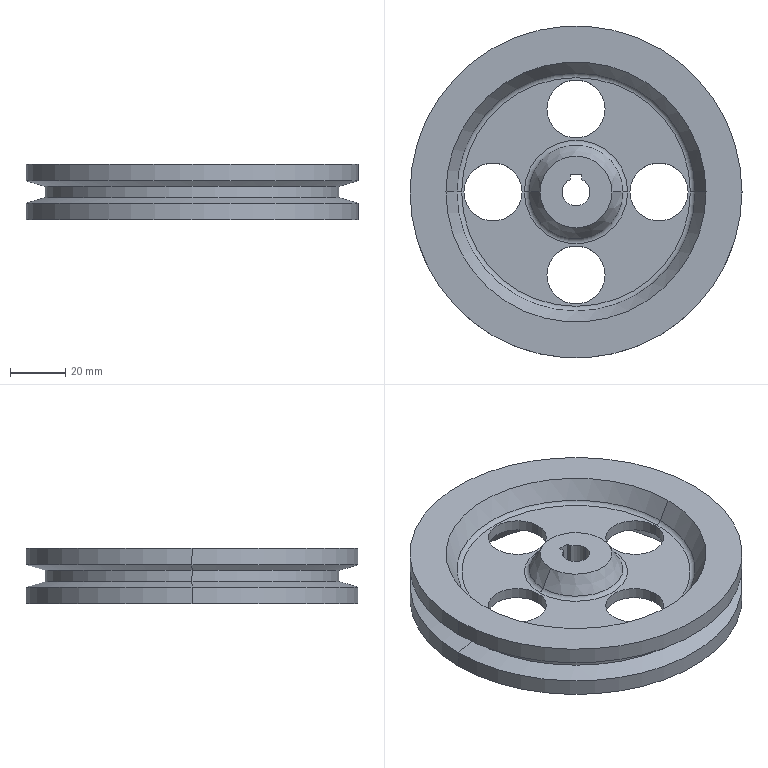Part | NX | features BREP 1 | 1 solid | 46 faces | box 120 x 120 x 20 mm | volume 115152 mm3 | cylinder 17 | cone 12 | plane 9 | torus 8 | commonest cylinder face diameters 21 x8 120 x4 10 x3 106 x2
STEP:
#1=CARTESIAN_POINT('',(-19.5,0.,-1.977));
#2=VERTEX_POINT('',#1);
#3=CARTESIAN_POINT('',(-40.5,0.,-1.977));
#4=VERTEX_POINT('',#3);
#5=CARTESIAN_POINT('',(-30.,0.,-1.977));
#6=DIRECTION('',(0.,0.,-1.));
#7=DIRECTION('',(-1.,0.,0.));
#8=AXIS2_PLACEMENT_3D('',#5,#6,#7);
#9=CIRCLE('',#8,10.5);
#10=EDGE_CURVE('',#2,#4,#9,.T.);
#11=ORIENTED_EDGE('',*,*,#10,.T.);
#12=CARTESIAN_POINT('',(-40.5,0.,2.023));
#13=VERTEX_POINT('',#12);
#14=CARTESIAN_POINT('',(-40.5,0.,-9.977));
#15=DIRECTION('',(0.,0.,1.));
#16=VECTOR('',#15,1000.);
#17=LINE('',#14,#16);
#18=EDGE_CURVE('',#4,#13,#17,.T.);
#19=ORIENTED_EDGE('',*,*,#18,.T.);
#20=CARTESIAN_POINT('',(-19.5,0.,2.023));
#21=VERTEX_POINT('',#20);
#22=CARTESIAN_POINT('',(-30.,0.,2.023));
#23=DIRECTION('',(0.,0.,1.));
#24=DIRECTION('',(1.,0.,0.));
#25=AXIS2_PLACEMENT_3D('',#22,#23,#24);
#26=CIRCLE('',#25,10.5);
#27=EDGE_CURVE('',#13,#21,#26,.T.);
#28=ORIENTED_EDGE('',*,*,#27,.T.);
#29=CARTESIAN_POINT('',(-19.5,0.,-9.977));
#30=DIRECTION('',(0.,0.,1.));
#31=VECTOR('',#30,1000.);
#32=LINE('',#29,#31);
#33=EDGE_CURVE('',#2,#21,#32,.T.);
#34=ORIENTED_EDGE('',*,*,#33,.F.);
#35=EDGE_LOOP('',(#11,#19,#28,#34));
#36=FACE_BOUND('',#35,.T.);
#37=CARTESIAN_POINT('',(-30.,0.,-9.977));
#38=DIRECTION('',(0.,0.,1.));
#39=DIRECTION('',(-1.,0.,0.));
#40=AXIS2_PLACEMENT_3D('',#37,#38,#39);
#41=CYLINDRICAL_SURFACE('',#40,10.5);
#42=ADVANCED_FACE('',(#36),#41,.F.);
#43=CARTESIAN_POINT('',(10.5,-30.,-1.977));
#44=VERTEX_POINT('',#43);
#45=CARTESIAN_POINT('',(-10.5,-30.,-1.977));
#46=VERTEX_POINT('',#45);
#47=CARTESIAN_POINT('',(0.,-30.,-1.977));
#48=DIRECTION('',(0.,0.,-1.));
#49=DIRECTION('',(-1.,0.,0.));
#50=AXIS2_PLACEMENT_3D('',#47,#48,#49);
#51=CIRCLE('',#50,10.5);
#52=EDGE_CURVE('',#44,#46,#51,.T.);
#53=ORIENTED_EDGE('',*,*,#52,.T.);
#54=CARTESIAN_POINT('',(-10.5,-30.,2.023));
#55=VERTEX_POINT('',#54);
#56=CARTESIAN_POINT('',(-10.5,-30.,-9.977));
#57=DIRECTION('',(0.,0.,1.));
#58=VECTOR('',#57,1000.);
#59=LINE('',#56,#58);
#60=EDGE_CURVE('',#46,#55,#59,.T.);
#61=ORIENTED_EDGE('',*,*,#60,.T.);
#62=CARTESIAN_POINT('',(10.5,-30.,2.023));
#63=VERTEX_POINT('',#62);
#64=CARTESIAN_POINT('',(0.,-30.,2.023));
#65=DIRECTION('',(0.,0.,1.));
#66=DIRECTION('',(1.,0.,0.));
#67=AXIS2_PLACEMENT_3D('',#64,#65,#66);
#68=CIRCLE('',#67,10.5);
#69=EDGE_CURVE('',#55,#63,#68,.T.);
#70=ORIENTED_EDGE('',*,*,#69,.T.);
#71=CARTESIAN_POINT('',(10.5,-30.,-9.977));
#72=DIRECTION('',(0.,0.,1.));
#73=VECTOR('',#72,1000.);
#74=LINE('',#71,#73);
#75=EDGE_CURVE('',#44,#63,#74,.T.);
#76=ORIENTED_EDGE('',*,*,#75,.F.);
#77=EDGE_LOOP('',(#53,#61,#70,#76));
#78=FACE_BOUND('',#77,.T.);
#79=CARTESIAN_POINT('',(0.,-30.,-9.977));
#80=DIRECTION('',(0.,0.,1.));
#81=DIRECTION('',(-1.,0.,0.));
#82=AXIS2_PLACEMENT_3D('',#79,#80,#81);
#83=CYLINDRICAL_SURFACE('',#82,10.5);
#84=ADVANCED_FACE('',(#78),#83,.F.);
#85=CARTESIAN_POINT('',(40.5,0.,-1.977));
#86=VERTEX_POINT('',#85);
#87=CARTESIAN_POINT('',(19.5,0.,-1.977));
#88=VERTEX_POINT('',#87);
#89=CARTESIAN_POINT('',(30.,0.,-1.977));
#90=DIRECTION('',(0.,0.,-1.));
#91=DIRECTION('',(-1.,0.,0.));
#92=AXIS2_PLACEMENT_3D('',#89,#90,#91);
#93=CIRCLE('',#92,10.5);
#94=EDGE_CURVE('',#86,#88,#93,.T.);
#95=ORIENTED_EDGE('',*,*,#94,.T.);
#96=CARTESIAN_POINT('',(19.5,0.,2.023));
#97=VERTEX_POINT('',#96);
#98=CARTESIAN_POINT('',(19.5,0.,-9.977));
#99=DIRECTION('',(0.,0.,1.));
#100=VECTOR('',#99,1000.);
#101=LINE('',#98,#100);
#102=EDGE_CURVE('',#88,#97,#101,.T.);
#103=ORIENTED_EDGE('',*,*,#102,.T.);
#104=CARTESIAN_POINT('',(40.5,0.,2.023));
#105=VERTEX_POINT('',#104);
#106=CARTESIAN_POINT('',(30.,0.,2.023));
#107=DIRECTION('',(0.,0.,1.));
#108=DIRECTION('',(1.,0.,0.));
#109=AXIS2_PLACEMENT_3D('',#106,#107,#108);
#110=CIRCLE('',#109,10.5);
#111=EDGE_CURVE('',#97,#105,#110,.T.);
#112=ORIENTED_EDGE('',*,*,#111,.T.);
#113=CARTESIAN_POINT('',(40.5,0.,-9.977));
#114=DIRECTION('',(0.,0.,1.));
#115=VECTOR('',#114,1000.);
#116=LINE('',#113,#115);
#117=EDGE_CURVE('',#86,#105,#116,.T.);
#118=ORIENTED_EDGE('',*,*,#117,.F.);
#119=EDGE_LOOP('',(#95,#103,#112,#118));
#120=FACE_BOUND('',#119,.T.);
#121=CARTESIAN_POINT('',(30.,0.,-9.977));
#122=DIRECTION('',(0.,0.,1.));
#123=DIRECTION('',(-1.,0.,0.));
#124=AXIS2_PLACEMENT_3D('',#121,#122,#123);
#125=CYLINDRICAL_SURFACE('',#124,10.5);
#126=ADVANCED_FACE('',(#120),#125,.F.);
#127=CARTESIAN_POINT('',(10.5,30.,-1.977));
#128=VERTEX_POINT('',#127);
#129=CARTESIAN_POINT('',(-10.5,30.,-1.977));
#130=VERTEX_POINT('',#129);
#131=CARTESIAN_POINT('',(0.,30.,-1.977));
#132=DIRECTION('',(0.,0.,-1.));
#133=DIRECTION('',(-1.,0.,0.));
#134=AXIS2_PLACEMENT_3D('',#131,#132,#133);
#135=CIRCLE('',#134,10.5);
#136=EDGE_CURVE('',#128,#130,#135,.T.);
#137=ORIENTED_EDGE('',*,*,#136,.T.);
#138=CARTESIAN_POINT('',(-10.5,30.,2.023));
#139=VERTEX_POINT('',#138);
#140=CARTESIAN_POINT('',(-10.5,30.,-9.977));
#141=DIRECTION('',(0.,0.,1.));
#142=VECTOR('',#141,1000.);
#143=LINE('',#140,#142);
#144=EDGE_CURVE('',#130,#139,#143,.T.);
#145=ORIENTED_EDGE('',*,*,#144,.T.);
#146=CARTESIAN_POINT('',(10.5,30.,2.023));
#147=VERTEX_POINT('',#146);
#148=CARTESIAN_POINT('',(0.,30.,2.023));
#149=DIRECTION('',(0.,0.,1.));
#150=DIRECTION('',(1.,0.,0.));
#151=AXIS2_PLACEMENT_3D('',#148,#149,#150);
#152=CIRCLE('',#151,10.5);
#153=EDGE_CURVE('',#139,#147,#152,.T.);
#154=ORIENTED_EDGE('',*,*,#153,.T.);
#155=CARTESIAN_POINT('',(10.5,30.,-9.977));
#156=DIRECTION('',(0.,0.,1.));
#157=VECTOR('',#156,1000.);
#158=LINE('',#155,#157);
#159=EDGE_CURVE('',#128,#147,#158,.T.);
#160=ORIENTED_EDGE('',*,*,#159,.F.);
#161=EDGE_LOOP('',(#137,#145,#154,#160));
#162=FACE_BOUND('',#161,.T.);
#163=CARTESIAN_POINT('',(0.,30.,-9.977));
#164=DIRECTION('',(0.,0.,1.));
#165=DIRECTION('',(-1.,0.,0.));
#166=AXIS2_PLACEMENT_3D('',#163,#164,#165);
#167=CYLINDRICAL_SURFACE('',#166,10.5);
#168=ADVANCED_FACE('',(#162),#167,.F.);
#169=CARTESIAN_POINT('',(13.,0.,10.023));
#170=VERTEX_POINT('',#169);
#171=CARTESIAN_POINT('',(-13.,0.,10.023));
#172=VERTEX_POINT('',#171);
#173=CARTESIAN_POINT('',(0.,0.,10.023));
#174=DIRECTION('',(0.,0.,1.));
#175=DIRECTION('',(1.,0.,0.));
#176=AXIS2_PLACEMENT_3D('',#173,#174,#175);
#177=CIRCLE('',#176,13.);
#178=EDGE_CURVE('',#170,#172,#177,.T.);
#179=ORIENTED_EDGE('',*,*,#178,.F.);
#180=CARTESIAN_POINT('',(16.927,0.,3.042));
#181=VERTEX_POINT('',#180);
#182=CARTESIAN_POINT('',(13.,0.,10.023));
#183=DIRECTION('',(0.4903,0.,-0.8716));
#184=VECTOR('',#183,1000.);
#185=LINE('',#182,#184);
#186=EDGE_CURVE('',#181,#170,#185,.F.);
#187=ORIENTED_EDGE('',*,*,#186,.F.);
#188=CARTESIAN_POINT('',(-16.927,0.,3.042));
#189=VERTEX_POINT('',#188);
#190=CARTESIAN_POINT('',(0.,0.,3.042));
#191=DIRECTION('',(0.,0.,1.));
#192=DIRECTION('',(1.,0.,0.));
#193=AXIS2_PLACEMENT_3D('',#190,#191,#192);
#194=CIRCLE('',#193,16.927);
#195=EDGE_CURVE('',#181,#189,#194,.T.);
#196=ORIENTED_EDGE('',*,*,#195,.T.);
#197=CARTESIAN_POINT('',(-13.,0.,10.023));
#198=DIRECTION('',(-0.4903,0.,-0.8716));
#199=VECTOR('',#198,1000.);
#200=LINE('',#197,#199);
#201=EDGE_CURVE('',#189,#172,#200,.F.);
#202=ORIENTED_EDGE('',*,*,#201,.T.);
#203=EDGE_LOOP('',(#179,#187,#196,#202));
#204=FACE_BOUND('',#203,.T.);
#205=CARTESIAN_POINT('',(0.,0.,10.023));
#206=DIRECTION('',(0.,0.,-1.));
#207=DIRECTION('',(1.,0.,0.));
#208=AXIS2_PLACEMENT_3D('',#205,#206,#207);
#209=CONICAL_SURFACE('',#208,13.,0.5124);
#210=ADVANCED_FACE('',(#204),#209,.T.);
#211=CARTESIAN_POINT('',(0.,0.,3.042));
#212=DIRECTION('',(0.,0.,1.));
#213=DIRECTION('',(1.,0.,0.));
#214=AXIS2_PLACEMENT_3D('',#211,#212,#213);
#215=CIRCLE('',#214,16.927);
#216=EDGE_CURVE('',#189,#181,#215,.T.);
#217=ORIENTED_EDGE('',*,*,#216,.F.);
#218=CARTESIAN_POINT('',(-18.67,0.,2.023));
#219=VERTEX_POINT('',#218);
#220=CARTESIAN_POINT('',(-18.67,0.,4.023));
#221=DIRECTION('',(0.,1.,0.));
#222=DIRECTION('',(-1.,0.,0.));
#223=AXIS2_PLACEMENT_3D('',#220,#221,#222);
#224=CIRCLE('',#223,2.);
#225=EDGE_CURVE('',#189,#219,#224,.T.);
#226=ORIENTED_EDGE('',*,*,#225,.T.);
#227=CARTESIAN_POINT('',(18.67,0.,2.023));
#228=VERTEX_POINT('',#227);
#229=CARTESIAN_POINT('',(0.,0.,2.023));
#230=DIRECTION('',(0.,0.,1.));
#231=DIRECTION('',(1.,0.,0.));
#232=AXIS2_PLACEMENT_3D('',#229,#230,#231);
#233=CIRCLE('',#232,18.67);
#234=EDGE_CURVE('',#219,#228,#233,.T.);
#235=ORIENTED_EDGE('',*,*,#234,.T.);
#236=CARTESIAN_POINT('',(18.67,0.,4.023));
#237=DIRECTION('',(0.,-1.,0.));
#238=DIRECTION('',(0.,0.,-1.));
#239=AXIS2_PLACEMENT_3D('',#236,#237,#238);
#240=CIRCLE('',#239,2.);
#241=EDGE_CURVE('',#181,#228,#240,.T.);
#242=ORIENTED_EDGE('',*,*,#241,.F.);
#243=EDGE_LOOP('',(#217,#226,#235,#242));
#244=FACE_BOUND('',#243,.T.);
#245=CARTESIAN_POINT('',(0.,0.,4.023));
#246=DIRECTION('',(0.,0.,1.));
#247=DIRECTION('',(-1.,0.,0.));
#248=AXIS2_PLACEMENT_3D('',#245,#246,#247);
#249=TOROIDAL_SURFACE('',#248,18.67,2.);
#250=ADVANCED_FACE('',(#244),#249,.F.);
#251=CARTESIAN_POINT('',(-41.33,0.,2.023));
#252=VERTEX_POINT('',#251);
#253=CARTESIAN_POINT('',(41.33,0.,2.023));
#254=VERTEX_POINT('',#253);
#255=CARTESIAN_POINT('',(0.,0.,2.023));
#256=DIRECTION('',(0.,0.,1.));
#257=DIRECTION('',(1.,0.,0.));
#258=AXIS2_PLACEMENT_3D('',#255,#256,#257);
#259=CIRCLE('',#258,41.33);
#260=EDGE_CURVE('',#252,#254,#259,.T.);
#261=ORIENTED_EDGE('',*,*,#260,.F.);
#262=CARTESIAN_POINT('',(-43.073,0.,3.042));
#263=VERTEX_POINT('',#262);
#264=CARTESIAN_POINT('',(-41.33,0.,4.023));
#265=DIRECTION('',(0.,1.,0.));
#266=DIRECTION('',(-1.,0.,0.));
#267=AXIS2_PLACEMENT_3D('',#264,#265,#266);
#268=CIRCLE('',#267,2.);
#269=EDGE_CURVE('',#252,#263,#268,.T.);
#270=ORIENTED_EDGE('',*,*,#269,.T.);
#271=CARTESIAN_POINT('',(43.073,0.,3.042));
#272=VERTEX_POINT('',#271);
#273=CARTESIAN_POINT('',(0.,0.,3.042));
#274=DIRECTION('',(0.,0.,1.));
#275=DIRECTION('',(1.,0.,0.));
#276=AXIS2_PLACEMENT_3D('',#273,#274,#275);
#277=CIRCLE('',#276,43.073);
#278=EDGE_CURVE('',#263,#272,#277,.T.);
#279=ORIENTED_EDGE('',*,*,#278,.T.);
#280=CARTESIAN_POINT('',(41.33,0.,4.023));
#281=DIRECTION('',(0.,-1.,0.));
#282=DIRECTION('',(0.,0.,-1.));
#283=AXIS2_PLACEMENT_3D('',#280,#281,#282);
#284=CIRCLE('',#283,2.);
#285=EDGE_CURVE('',#254,#272,#284,.T.);
#286=ORIENTED_EDGE('',*,*,#285,.F.);
#287=EDGE_LOOP('',(#261,#270,#279,#286));
#288=FACE_BOUND('',#287,.T.);
#289=CARTESIAN_POINT('',(0.,0.,4.023));
#290=DIRECTION('',(0.,0.,1.));
#291=DIRECTION('',(-1.,0.,0.));
#292=AXIS2_PLACEMENT_3D('',#289,#290,#291);
#293=TOROIDAL_SURFACE('',#292,41.33,2.);
#294=ADVANCED_FACE('',(#288),#293,.F.);
#295=ORIENTED_EDGE('',*,*,#278,.F.);
#296=CARTESIAN_POINT('',(-47.,0.,10.023));
#297=VERTEX_POINT('',#296);
#298=CARTESIAN_POINT('',(-43.073,0.,3.042));
#299=DIRECTION('',(-0.4903,0.,0.8716));
#300=VECTOR('',#299,1000.);
#301=LINE('',#298,#300);
#302=EDGE_CURVE('',#263,#297,#301,.T.);
#303=ORIENTED_EDGE('',*,*,#302,.T.);
#304=CARTESIAN_POINT('',(47.,0.,10.023));
#305=VERTEX_POINT('',#304);
#306=CARTESIAN_POINT('',(0.,0.,10.023));
#307=DIRECTION('',(0.,0.,1.));
#308=DIRECTION('',(1.,0.,0.));
#309=AXIS2_PLACEMENT_3D('',#306,#307,#308);
#310=CIRCLE('',#309,47.);
#311=EDGE_CURVE('',#297,#305,#310,.T.);
#312=ORIENTED_EDGE('',*,*,#311,.T.);
#313=CARTESIAN_POINT('',(43.073,0.,3.042));
#314=DIRECTION('',(0.4903,0.,0.8716));
#315=VECTOR('',#314,1000.);
#316=LINE('',#313,#315);
#317=EDGE_CURVE('',#272,#305,#316,.T.);
#318=ORIENTED_EDGE('',*,*,#317,.F.);
#319=EDGE_LOOP('',(#295,#303,#312,#318));
#320=FACE_BOUND('',#319,.T.);
#321=CARTESIAN_POINT('',(0.,0.,3.042));
#322=DIRECTION('',(0.,0.,1.));
#323=DIRECTION('',(-1.,0.,0.));
#324=AXIS2_PLACEMENT_3D('',#321,#322,#323);
#325=CONICAL_SURFACE('',#324,43.073,0.5124);
#326=ADVANCED_FACE('',(#320),#325,.F.);
#327=CARTESIAN_POINT('',(60.,0.,4.023));
#328=VERTEX_POINT('',#327);
#329=CARTESIAN_POINT('',(-60.,0.,4.023));
#330=VERTEX_POINT('',#329);
#331=CARTESIAN_POINT('',(0.,0.,4.023));
#332=DIRECTION('',(0.,0.,1.));
#333=DIRECTION('',(1.,0.,0.));
#334=AXIS2_PLACEMENT_3D('',#331,#332,#333);
#335=CIRCLE('',#334,60.);
#336=EDGE_CURVE('',#328,#330,#335,.T.);
#337=ORIENTED_EDGE('',*,*,#336,.T.);
#338=CARTESIAN_POINT('',(-60.,0.,10.023));
#339=VERTEX_POINT('',#338);
#340=CARTESIAN_POINT('',(-60.,0.,55.569));
#341=DIRECTION('',(0.,0.,1.));
#342=VECTOR('',#341,1000.);
#343=LINE('',#340,#342);
#344=EDGE_CURVE('',#330,#339,#343,.T.);
#345=ORIENTED_EDGE('',*,*,#344,.T.);
#346=CARTESIAN_POINT('',(60.,0.,10.023));
#347=VERTEX_POINT('',#346);
#348=CARTESIAN_POINT('',(0.,0.,10.023));
#349=DIRECTION('',(0.,0.,1.));
#350=DIRECTION('',(1.,0.,0.));
#351=AXIS2_PLACEMENT_3D('',#348,#349,#350);
#352=CIRCLE('',#351,60.);
#353=EDGE_CURVE('',#347,#339,#352,.T.);
#354=ORIENTED_EDGE('',*,*,#353,.F.);
#355=CARTESIAN_POINT('',(60.,0.,55.569));
#356=DIRECTION('',(0.,0.,1.));
#357=VECTOR('',#356,1000.);
#358=LINE('',#355,#357);
#359=EDGE_CURVE('',#328,#347,#358,.T.);
#360=ORIENTED_EDGE('',*,*,#359,.F.);
#361=EDGE_LOOP('',(#337,#345,#354,#360));
#362=FACE_BOUND('',#361,.T.);
#363=CARTESIAN_POINT('',(0.,0.,55.569));
#364=DIRECTION('',(0.,0.,1.));
#365=DIRECTION('',(-1.,0.,0.));
#366=AXIS2_PLACEMENT_3D('',#363,#364,#365);
#367=CYLINDRICAL_SURFACE('',#366,60.);
#368=ADVANCED_FACE('',(#362),#367,.T.);
#369=CARTESIAN_POINT('',(53.,0.,2.023));
#370=VERTEX_POINT('',#369);
#371=CARTESIAN_POINT('',(-53.,0.,2.023));
#372=VERTEX_POINT('',#371);
#373=CARTESIAN_POINT('',(0.,0.,2.023));
#374=DIRECTION('',(0.,0.,1.));
#375=DIRECTION('',(1.,0.,0.));
#376=AXIS2_PLACEMENT_3D('',#373,#374,#375);
#377=CIRCLE('',#376,53.);
#378=EDGE_CURVE('',#370,#372,#377,.T.);
#379=ORIENTED_EDGE('',*,*,#378,.T.);
#380=CARTESIAN_POINT('',(-60.,0.,4.023));
#381=DIRECTION('',(-0.9615,0.,0.2747));
#382=VECTOR('',#381,1000.);
#383=LINE('',#380,#382);
#384=EDGE_CURVE('',#372,#330,#383,.T.);
#385=ORIENTED_EDGE('',*,*,#384,.T.);
#386=ORIENTED_EDGE('',*,*,#336,.F.);
#387=CARTESIAN_POINT('',(60.,0.,4.023));
#388=DIRECTION('',(0.9615,0.,0.2747));
#389=VECTOR('',#388,1000.);
#390=LINE('',#387,#389);
#391=EDGE_CURVE('',#370,#328,#390,.T.);
#392=ORIENTED_EDGE('',*,*,#391,.F.);
#393=EDGE_LOOP('',(#379,#385,#386,#392));
#394=FACE_BOUND('',#393,.T.);
#395=CARTESIAN_POINT('',(0.,0.,4.023));
#396=DIRECTION('',(0.,0.,1.));
#397=DIRECTION('',(-1.,0.,0.));
#398=AXIS2_PLACEMENT_3D('',#395,#396,#397);
#399=CONICAL_SURFACE('',#398,60.,1.292);
#400=ADVANCED_FACE('',(#394),#399,.T.);
#401=CARTESIAN_POINT('',(53.,0.,-1.977));
#402=VERTEX_POINT('',#401);
#403=CARTESIAN_POINT('',(-53.,0.,-1.977));
#404=VERTEX_POINT('',#403);
#405=CARTESIAN_POINT('',(0.,0.,-1.977));
#406=DIRECTION('',(0.,0.,1.));
#407=DIRECTION('',(1.,0.,0.));
#408=AXIS2_PLACEMENT_3D('',#405,#406,#407);
#409=CIRCLE('',#408,53.);
#410=EDGE_CURVE('',#402,#404,#409,.T.);
#411=ORIENTED_EDGE('',*,*,#410,.T.);
#412=CARTESIAN_POINT('',(-53.,0.,55.569));
#413=DIRECTION('',(0.,0.,1.));
#414=VECTOR('',#413,1000.);
#415=LINE('',#412,#414);
#416=EDGE_CURVE('',#404,#372,#415,.T.);
#417=ORIENTED_EDGE('',*,*,#416,.T.);
#418=ORIENTED_EDGE('',*,*,#378,.F.);
#419=CARTESIAN_POINT('',(53.,0.,55.569));
#420=DIRECTION('',(0.,0.,1.));
#421=VECTOR('',#420,1000.);
#422=LINE('',#419,#421);
#423=EDGE_CURVE('',#402,#370,#422,.T.);
#424=ORIENTED_EDGE('',*,*,#423,.F.);
#425=EDGE_LOOP('',(#411,#417,#418,#424));
#426=FACE_BOUND('',#425,.T.);
#427=CARTESIAN_POINT('',(0.,0.,55.569));
#428=DIRECTION('',(0.,0.,1.));
#429=DIRECTION('',(-1.,0.,0.));
#430=AXIS2_PLACEMENT_3D('',#427,#428,#429);
#431=CYLINDRICAL_SURFACE('',#430,53.);
#432=ADVANCED_FACE('',(#426),#431,.T.);
#433=ORIENTED_EDGE('',*,*,#410,.F.);
#434=CARTESIAN_POINT('',(60.,0.,-3.977));
#435=VERTEX_POINT('',#434);
#436=CARTESIAN_POINT('',(53.,0.,-1.977));
#437=DIRECTION('',(0.9615,0.,-0.2747));
#438=VECTOR('',#437,1000.);
#439=LINE('',#436,#438);
#440=EDGE_CURVE('',#435,#402,#439,.F.);
#441=ORIENTED_EDGE('',*,*,#440,.F.);
#442=CARTESIAN_POINT('',(-60.,0.,-3.977));
#443=VERTEX_POINT('',#442);
#444=CARTESIAN_POINT('',(0.,0.,-3.977));
#445=DIRECTION('',(0.,0.,1.));
#446=DIRECTION('',(1.,0.,0.));
#447=AXIS2_PLACEMENT_3D('',#444,#445,#446);
#448=CIRCLE('',#447,60.);
#449=EDGE_CURVE('',#435,#443,#448,.T.);
#450=ORIENTED_EDGE('',*,*,#449,.T.);
#451=CARTESIAN_POINT('',(-53.,0.,-1.977));
#452=DIRECTION('',(-0.9615,0.,-0.2747));
#453=VECTOR('',#452,1000.);
#454=LINE('',#451,#453);
#455=EDGE_CURVE('',#443,#404,#454,.F.);
#456=ORIENTED_EDGE('',*,*,#455,.T.);
#457=EDGE_LOOP('',(#433,#441,#450,#456));
#458=FACE_BOUND('',#457,.T.);
#459=CARTESIAN_POINT('',(0.,0.,-1.977));
#460=DIRECTION('',(0.,0.,-1.));
#461=DIRECTION('',(1.,0.,0.));
#462=AXIS2_PLACEMENT_3D('',#459,#460,#461);
#463=CONICAL_SURFACE('',#462,53.,1.292);
#464=ADVANCED_FACE('',(#458),#463,.T.);
#465=CARTESIAN_POINT('',(60.,0.,-9.977));
#466=VERTEX_POINT('',#465);
#467=CARTESIAN_POINT('',(-60.,0.,-9.977));
#468=VERTEX_POINT('',#467);
#469=CARTESIAN_POINT('',(0.,0.,-9.977));
#470=DIRECTION('',(0.,0.,1.));
#471=DIRECTION('',(1.,0.,0.));
#472=AXIS2_PLACEMENT_3D('',#469,#470,#471);
#473=CIRCLE('',#472,60.);
#474=EDGE_CURVE('',#466,#468,#473,.T.);
#475=ORIENTED_EDGE('',*,*,#474,.T.);
#476=CARTESIAN_POINT('',(-60.,0.,55.569));
#477=DIRECTION('',(0.,0.,1.));
#478=VECTOR('',#477,1000.);
#479=LINE('',#476,#478);
#480=EDGE_CURVE('',#468,#443,#479,.T.);
#481=ORIENTED_EDGE('',*,*,#480,.T.);
#482=ORIENTED_EDGE('',*,*,#449,.F.);
#483=CARTESIAN_POINT('',(60.,0.,55.569));
#484=DIRECTION('',(0.,0.,1.));
#485=VECTOR('',#484,1000.);
#486=LINE('',#483,#485);
#487=EDGE_CURVE('',#466,#435,#486,.T.);
#488=ORIENTED_EDGE('',*,*,#487,.F.);
#489=EDGE_LOOP('',(#475,#481,#482,#488));
#490=FACE_BOUND('',#489,.T.);
#491=CARTESIAN_POINT('',(0.,0.,55.569));
#492=DIRECTION('',(0.,0.,1.));
#493=DIRECTION('',(-1.,0.,0.));
#494=AXIS2_PLACEMENT_3D('',#491,#492,#493);
#495=CYLINDRICAL_SURFACE('',#494,60.);
#496=ADVANCED_FACE('',(#490),#495,.T.);
#497=CARTESIAN_POINT('',(-43.073,0.,-2.997));
#498=VERTEX_POINT('',#497);
#499=CARTESIAN_POINT('',(43.073,0.,-2.997));
#500=VERTEX_POINT('',#499);
#501=CARTESIAN_POINT('',(0.,0.,-2.997));
#502=DIRECTION('',(0.,0.,1.));
#503=DIRECTION('',(1.,0.,0.));
#504=AXIS2_PLACEMENT_3D('',#501,#502,#503);
#505=CIRCLE('',#504,43.073);
#506=EDGE_CURVE('',#498,#500,#505,.T.);
#507=ORIENTED_EDGE('',*,*,#506,.T.);
#508=CARTESIAN_POINT('',(47.,0.,-9.977));
#509=VERTEX_POINT('',#508);
#510=CARTESIAN_POINT('',(47.,0.,-9.977));
#511=DIRECTION('',(0.4903,0.,-0.8716));
#512=VECTOR('',#511,1000.);
#513=LINE('',#510,#512);
#514=EDGE_CURVE('',#509,#500,#513,.F.);
#515=ORIENTED_EDGE('',*,*,#514,.F.);
#516=CARTESIAN_POINT('',(-47.,0.,-9.977));
#517=VERTEX_POINT('',#516);
#518=CARTESIAN_POINT('',(0.,0.,-9.977));
#519=DIRECTION('',(0.,0.,1.));
#520=DIRECTION('',(1.,0.,0.));
#521=AXIS2_PLACEMENT_3D('',#518,#519,#520);
#522=CIRCLE('',#521,47.);
#523=EDGE_CURVE('',#517,#509,#522,.T.);
#524=ORIENTED_EDGE('',*,*,#523,.F.);
#525=CARTESIAN_POINT('',(-47.,0.,-9.977));
#526=DIRECTION('',(-0.4903,0.,-0.8716));
#527=VECTOR('',#526,1000.);
#528=LINE('',#525,#527);
#529=EDGE_CURVE('',#517,#498,#528,.F.);
#530=ORIENTED_EDGE('',*,*,#529,.T.);
#531=EDGE_LOOP('',(#507,#515,#524,#530));
#532=FACE_BOUND('',#531,.T.);
#533=CARTESIAN_POINT('',(0.,0.,-9.977));
#534=DIRECTION('',(0.,0.,-1.));
#535=DIRECTION('',(1.,0.,0.));
#536=AXIS2_PLACEMENT_3D('',#533,#534,#535);
#537=CONICAL_SURFACE('',#536,47.,0.5124);
#538=ADVANCED_FACE('',(#532),#537,.F.);
#539=ORIENTED_EDGE('',*,*,#506,.F.);
#540=CARTESIAN_POINT('',(-41.33,0.,-1.977));
#541=VERTEX_POINT('',#540);
#542=CARTESIAN_POINT('',(-41.33,0.,-3.977));
#543=DIRECTION('',(0.,1.,0.));
#544=DIRECTION('',(-1.,0.,0.));
#545=AXIS2_PLACEMENT_3D('',#542,#543,#544);
#546=CIRCLE('',#545,2.);
#547=EDGE_CURVE('',#498,#541,#546,.T.);
#548=ORIENTED_EDGE('',*,*,#547,.T.);
#549=CARTESIAN_POINT('',(41.33,0.,-1.977));
#550=VERTEX_POINT('',#549);
#551=CARTESIAN_POINT('',(0.,0.,-1.977));
#552=DIRECTION('',(0.,0.,1.));
#553=DIRECTION('',(1.,0.,0.));
#554=AXIS2_PLACEMENT_3D('',#551,#552,#553);
#555=CIRCLE('',#554,41.33);
#556=EDGE_CURVE('',#541,#550,#555,.T.);
#557=ORIENTED_EDGE('',*,*,#556,.T.);
#558=CARTESIAN_POINT('',(41.33,0.,-3.977));
#559=DIRECTION('',(0.,-1.,0.));
#560=DIRECTION('',(0.,0.,-1.));
#561=AXIS2_PLACEMENT_3D('',#558,#559,#560);
#562=CIRCLE('',#561,2.);
#563=EDGE_CURVE('',#500,#550,#562,.T.);
#564=ORIENTED_EDGE('',*,*,#563,.F.);
#565=EDGE_LOOP('',(#539,#548,#557,#564));
#566=FACE_BOUND('',#565,.T.);
#567=CARTESIAN_POINT('',(0.,0.,-3.977));
#568=DIRECTION('',(0.,0.,1.));
#569=DIRECTION('',(-1.,0.,0.));
#570=AXIS2_PLACEMENT_3D('',#567,#568,#569);
#571=TOROIDAL_SURFACE('',#570,41.33,2.);
#572=ADVANCED_FACE('',(#566),#571,.F.);
#573=CARTESIAN_POINT('',(-18.67,0.,-1.977));
#574=VERTEX_POINT('',#573);
#575=CARTESIAN_POINT('',(18.67,0.,-1.977));
#576=VERTEX_POINT('',#575);
#577=CARTESIAN_POINT('',(0.,0.,-1.977));
#578=DIRECTION('',(0.,0.,1.));
#579=DIRECTION('',(1.,0.,0.));
#580=AXIS2_PLACEMENT_3D('',#577,#578,#579);
#581=CIRCLE('',#580,18.67);
#582=EDGE_CURVE('',#574,#576,#581,.T.);
#583=ORIENTED_EDGE('',*,*,#582,.F.);
#584=CARTESIAN_POINT('',(-16.927,0.,-2.997));
#585=VERTEX_POINT('',#584);
#586=CARTESIAN_POINT('',(-18.67,0.,-3.977));
#587=DIRECTION('',(0.,1.,0.));
#588=DIRECTION('',(-1.,0.,0.));
#589=AXIS2_PLACEMENT_3D('',#586,#587,#588);
#590=CIRCLE('',#589,2.);
#591=EDGE_CURVE('',#574,#585,#590,.T.);
#592=ORIENTED_EDGE('',*,*,#591,.T.);
#593=CARTESIAN_POINT('',(16.927,0.,-2.997));
#594=VERTEX_POINT('',#593);
#595=CARTESIAN_POINT('',(0.,0.,-2.997));
#596=DIRECTION('',(0.,0.,1.));
#597=DIRECTION('',(1.,0.,0.));
#598=AXIS2_PLACEMENT_3D('',#595,#596,#597);
#599=CIRCLE('',#598,16.927);
#600=EDGE_CURVE('',#585,#594,#599,.T.);
#601=ORIENTED_EDGE('',*,*,#600,.T.);
#602=CARTESIAN_POINT('',(18.67,0.,-3.977));
#603=DIRECTION('',(0.,-1.,0.));
#604=DIRECTION('',(0.,0.,-1.));
#605=AXIS2_PLACEMENT_3D('',#602,#603,#604);
#606=CIRCLE('',#605,2.);
#607=EDGE_CURVE('',#576,#594,#606,.T.);
#608=ORIENTED_EDGE('',*,*,#607,.F.);
#609=EDGE_LOOP('',(#583,#592,#601,#608));
#610=FACE_BOUND('',#609,.T.);
#611=CARTESIAN_POINT('',(0.,0.,-3.977));
#612=DIRECTION('',(0.,0.,1.));
#613=DIRECTION('',(-1.,0.,0.));
#614=AXIS2_PLACEMENT_3D('',#611,#612,#613);
#615=TOROIDAL_SURFACE('',#614,18.67,2.);
#616=ADVANCED_FACE('',(#610),#615,.F.);
#617=CARTESIAN_POINT('',(13.,0.,-9.977));
#618=VERTEX_POINT('',#617);
#619=CARTESIAN_POINT('',(-13.,0.,-9.977));
#620=VERTEX_POINT('',#619);
#621=CARTESIAN_POINT('',(0.,0.,-9.977));
#622=DIRECTION('',(0.,0.,1.));
#623=DIRECTION('',(1.,0.,0.));
#624=AXIS2_PLACEMENT_3D('',#621,#622,#623);
#625=CIRCLE('',#624,13.);
#626=EDGE_CURVE('',#618,#620,#625,.T.);
#627=ORIENTED_EDGE('',*,*,#626,.T.);
#628=CARTESIAN_POINT('',(-16.927,0.,-2.997));
#629=DIRECTION('',(-0.4903,0.,0.8716));
#630=VECTOR('',#629,1000.);
#631=LINE('',#628,#630);
#632=EDGE_CURVE('',#620,#585,#631,.T.);
#633=ORIENTED_EDGE('',*,*,#632,.T.);
#634=CARTESIAN_POINT('',(0.,0.,-2.997));
#635=DIRECTION('',(0.,0.,1.));
#636=DIRECTION('',(1.,0.,0.));
#637=AXIS2_PLACEMENT_3D('',#634,#635,#636);
#638=CIRCLE('',#637,16.927);
#639=EDGE_CURVE('',#594,#585,#638,.T.);
#640=ORIENTED_EDGE('',*,*,#639,.F.);
#641=CARTESIAN_POINT('',(16.927,0.,-2.997));
#642=DIRECTION('',(0.4903,0.,0.8716));
#643=VECTOR('',#642,1000.);
#644=LINE('',#641,#643);
#645=EDGE_CURVE('',#618,#594,#644,.T.);
#646=ORIENTED_EDGE('',*,*,#645,.F.);
#647=EDGE_LOOP('',(#627,#633,#640,#646));
#648=FACE_BOUND('',#647,.T.);
#649=CARTESIAN_POINT('',(0.,0.,-2.997));
#650=DIRECTION('',(0.,0.,1.));
#651=DIRECTION('',(-1.,0.,0.));
#652=AXIS2_PLACEMENT_3D('',#649,#650,#651);
#653=CONICAL_SURFACE('',#652,16.927,0.5124);
#654=ADVANCED_FACE('',(#648),#653,.T.);
#655=CARTESIAN_POINT('',(-5.,0.,-9.977));
#656=VERTEX_POINT('',#655);
#657=CARTESIAN_POINT('',(5.,0.,-9.977));
#658=VERTEX_POINT('',#657);
#659=CARTESIAN_POINT('',(0.,0.,-9.977));
#660=DIRECTION('',(0.,0.,1.));
#661=DIRECTION('',(1.,0.,0.));
#662=AXIS2_PLACEMENT_3D('',#659,#660,#661);
#663=CIRCLE('',#662,5.);
#664=EDGE_CURVE('',#656,#658,#663,.T.);
#665=ORIENTED_EDGE('',*,*,#664,.F.);
#666=CARTESIAN_POINT('',(-5.,0.,10.023));
#667=VERTEX_POINT('',#666);
#668=CARTESIAN_POINT('',(-5.,0.,55.569));
#669=DIRECTION('',(0.,0.,1.));
#670=VECTOR('',#669,1000.);
#671=LINE('',#668,#670);
#672=EDGE_CURVE('',#656,#667,#671,.T.);
#673=ORIENTED_EDGE('',*,*,#672,.T.);
#674=CARTESIAN_POINT('',(5.,0.,10.023));
#675=VERTEX_POINT('',#674);
#676=CARTESIAN_POINT('',(0.,0.,10.023));
#677=DIRECTION('',(0.,0.,1.));
#678=DIRECTION('',(1.,0.,0.));
#679=AXIS2_PLACEMENT_3D('',#676,#677,#678);
#680=CIRCLE('',#679,5.);
#681=EDGE_CURVE('',#667,#675,#680,.T.);
#682=ORIENTED_EDGE('',*,*,#681,.T.);
#683=CARTESIAN_POINT('',(5.,0.,55.569));
#684=DIRECTION('',(0.,0.,1.));
#685=VECTOR('',#684,1000.);
#686=LINE('',#683,#685);
#687=EDGE_CURVE('',#658,#675,#686,.T.);
#688=ORIENTED_EDGE('',*,*,#687,.F.);
#689=EDGE_LOOP('',(#665,#673,#682,#688));
#690=FACE_BOUND('',#689,.T.);
#691=CARTESIAN_POINT('',(0.,0.,55.569));
#692=DIRECTION('',(0.,0.,1.));
#693=DIRECTION('',(-1.,0.,0.));
#694=AXIS2_PLACEMENT_3D('',#691,#692,#693);
#695=CYLINDRICAL_SURFACE('',#694,5.);
#696=ADVANCED_FACE('',(#690),#695,.F.);
#697=CARTESIAN_POINT('',(2.,4.583,-9.977));
#698=VERTEX_POINT('',#697);
#699=CARTESIAN_POINT('',(0.,0.,-9.977));
#700=DIRECTION('',(0.,0.,1.));
#701=DIRECTION('',(1.,0.,0.));
#702=AXIS2_PLACEMENT_3D('',#699,#700,#701);
#703=CIRCLE('',#702,5.);
#704=EDGE_CURVE('',#658,#698,#703,.T.);
#705=ORIENTED_EDGE('',*,*,#704,.F.);
#706=ORIENTED_EDGE('',*,*,#687,.T.);
#707=CARTESIAN_POINT('',(2.,4.583,10.023));
#708=VERTEX_POINT('',#707);
#709=CARTESIAN_POINT('',(0.,0.,10.023));
#710=DIRECTION('',(0.,0.,1.));
#711=DIRECTION('',(1.,0.,0.));
#712=AXIS2_PLACEMENT_3D('',#709,#710,#711);
#713=CIRCLE('',#712,5.);
#714=EDGE_CURVE('',#675,#708,#713,.T.);
#715=ORIENTED_EDGE('',*,*,#714,.T.);
#716=CARTESIAN_POINT('',(2.,4.583,10.023));
#717=DIRECTION('',(0.,0.,-1.));
#718=VECTOR('',#717,1000.);
#719=LINE('',#716,#718);
#720=EDGE_CURVE('',#708,#698,#719,.T.);
#721=ORIENTED_EDGE('',*,*,#720,.T.);
#722=EDGE_LOOP('',(#705,#706,#715,#721));
#723=FACE_BOUND('',#722,.T.);
#724=CARTESIAN_POINT('',(0.,0.,55.569));
#725=DIRECTION('',(0.,0.,1.));
#726=DIRECTION('',(-1.,0.,0.));
#727=AXIS2_PLACEMENT_3D('',#724,#725,#726);
#728=CYLINDRICAL_SURFACE('',#727,5.);
#729=ADVANCED_FACE('',(#723),#728,.F.);
#730=CARTESIAN_POINT('',(0.,0.,10.023));
#731=DIRECTION('',(0.,0.,1.));
#732=DIRECTION('',(1.,0.,0.));
#733=AXIS2_PLACEMENT_3D('',#730,#731,#732);
#734=CIRCLE('',#733,13.);
#735=EDGE_CURVE('',#172,#170,#734,.T.);
#736=ORIENTED_EDGE('',*,*,#735,.T.);
#737=ORIENTED_EDGE('',*,*,#178,.T.);
#738=EDGE_LOOP('',(#736,#737));
#739=FACE_BOUND('',#738,.T.);
#740=CARTESIAN_POINT('',(2.,6.3,10.023));
#741=VERTEX_POINT('',#740);
#742=CARTESIAN_POINT('',(2.,4.583,10.023));
#743=DIRECTION('',(0.,-1.,0.));
#744=VECTOR('',#743,1000.);
#745=LINE('',#742,#744);
#746=EDGE_CURVE('',#741,#708,#745,.T.);
#747=ORIENTED_EDGE('',*,*,#746,.T.);
#748=ORIENTED_EDGE('',*,*,#714,.F.);
#749=ORIENTED_EDGE('',*,*,#681,.F.);
#750=CARTESIAN_POINT('',(-2.,4.583,10.023));
#751=VERTEX_POINT('',#750);
#752=CARTESIAN_POINT('',(0.,0.,10.023));
#753=DIRECTION('',(0.,0.,1.));
#754=DIRECTION('',(1.,0.,0.));
#755=AXIS2_PLACEMENT_3D('',#752,#753,#754);
#756=CIRCLE('',#755,5.);
#757=EDGE_CURVE('',#751,#667,#756,.T.);
#758=ORIENTED_EDGE('',*,*,#757,.F.);
#759=CARTESIAN_POINT('',(-2.,6.3,10.023));
#760=VERTEX_POINT('',#759);
#761=CARTESIAN_POINT('',(-2.,4.583,10.023));
#762=DIRECTION('',(0.,1.,0.));
#763=VECTOR('',#762,1000.);
#764=LINE('',#761,#763);
#765=EDGE_CURVE('',#751,#760,#764,.T.);
#766=ORIENTED_EDGE('',*,*,#765,.T.);
#767=CARTESIAN_POINT('',(-2.,6.3,10.023));
#768=DIRECTION('',(1.,0.,0.));
#769=VECTOR('',#768,1000.);
#770=LINE('',#767,#769);
#771=EDGE_CURVE('',#760,#741,#770,.T.);
#772=ORIENTED_EDGE('',*,*,#771,.T.);
#773=EDGE_LOOP('',(#747,#748,#749,#758,#766,#772));
#774=FACE_BOUND('',#773,.T.);
#775=CARTESIAN_POINT('',(0.,-13.,10.023));
#776=DIRECTION('',(0.,0.,1.));
#777=DIRECTION('',(0.,1.,0.));
#778=AXIS2_PLACEMENT_3D('',#775,#776,#777);
#779=PLANE('',#778);
#780=ADVANCED_FACE('',(#739,#774),#779,.T.);
#781=ORIENTED_EDGE('',*,*,#672,.F.);
#782=CARTESIAN_POINT('',(-2.,4.583,-9.977));
#783=VERTEX_POINT('',#782);
#784=CARTESIAN_POINT('',(0.,0.,-9.977));
#785=DIRECTION('',(0.,0.,1.));
#786=DIRECTION('',(1.,0.,0.));
#787=AXIS2_PLACEMENT_3D('',#784,#785,#786);
#788=CIRCLE('',#787,5.);
#789=EDGE_CURVE('',#783,#656,#788,.T.);
#790=ORIENTED_EDGE('',*,*,#789,.F.);
#791=CARTESIAN_POINT('',(-2.,4.583,10.023));
#792=DIRECTION('',(0.,0.,-1.));
#793=VECTOR('',#792,1000.);
#794=LINE('',#791,#793);
#795=EDGE_CURVE('',#751,#783,#794,.T.);
#796=ORIENTED_EDGE('',*,*,#795,.F.);
#797=ORIENTED_EDGE('',*,*,#757,.T.);
#798=EDGE_LOOP('',(#781,#790,#796,#797));
#799=FACE_BOUND('',#798,.T.);
#800=CARTESIAN_POINT('',(0.,0.,55.569));
#801=DIRECTION('',(0.,0.,1.));
#802=DIRECTION('',(-1.,0.,0.));
#803=AXIS2_PLACEMENT_3D('',#800,#801,#802);
#804=CYLINDRICAL_SURFACE('',#803,5.);
#805=ADVANCED_FACE('',(#799),#804,.F.);
#806=ORIENTED_EDGE('',*,*,#626,.F.);
#807=CARTESIAN_POINT('',(0.,0.,-9.977));
#808=DIRECTION('',(0.,0.,1.));
#809=DIRECTION('',(1.,0.,0.));
#810=AXIS2_PLACEMENT_3D('',#807,#808,#809);
#811=CIRCLE('',#810,13.);
#812=EDGE_CURVE('',#620,#618,#811,.T.);
#813=ORIENTED_EDGE('',*,*,#812,.F.);
#814=EDGE_LOOP('',(#806,#813));
#815=FACE_BOUND('',#814,.T.);
#816=CARTESIAN_POINT('',(2.,6.3,-9.977));
#817=VERTEX_POINT('',#816);
#818=CARTESIAN_POINT('',(2.,4.583,-9.977));
#819=DIRECTION('',(0.,-1.,0.));
#820=VECTOR('',#819,1000.);
#821=LINE('',#818,#820);
#822=EDGE_CURVE('',#817,#698,#821,.T.);
#823=ORIENTED_EDGE('',*,*,#822,.F.);
#824=CARTESIAN_POINT('',(-2.,6.3,-9.977));
#825=VERTEX_POINT('',#824);
#826=CARTESIAN_POINT('',(-2.,6.3,-9.977));
#827=DIRECTION('',(1.,0.,0.));
#828=VECTOR('',#827,1000.);
#829=LINE('',#826,#828);
#830=EDGE_CURVE('',#825,#817,#829,.T.);
#831=ORIENTED_EDGE('',*,*,#830,.F.);
#832=CARTESIAN_POINT('',(-2.,4.583,-9.977));
#833=DIRECTION('',(0.,1.,0.));
#834=VECTOR('',#833,1000.);
#835=LINE('',#832,#834);
#836=EDGE_CURVE('',#783,#825,#835,.T.);
#837=ORIENTED_EDGE('',*,*,#836,.F.);
#838=ORIENTED_EDGE('',*,*,#789,.T.);
#839=ORIENTED_EDGE('',*,*,#664,.T.);
#840=ORIENTED_EDGE('',*,*,#704,.T.);
#841=EDGE_LOOP('',(#823,#831,#837,#838,#839,#840));
#842=FACE_BOUND('',#841,.T.);
#843=CARTESIAN_POINT('',(0.,-13.,-9.977));
#844=DIRECTION('',(0.,0.,-1.));
#845=DIRECTION('',(1.,0.,0.));
#846=AXIS2_PLACEMENT_3D('',#843,#844,#845);
#847=PLANE('',#846);
#848=ADVANCED_FACE('',(#815,#842),#847,.T.);
#849=ORIENTED_EDGE('',*,*,#632,.F.);
#850=ORIENTED_EDGE('',*,*,#812,.T.);
#851=ORIENTED_EDGE('',*,*,#645,.T.);
#852=ORIENTED_EDGE('',*,*,#600,.F.);
#853=EDGE_LOOP('',(#849,#850,#851,#852));
#854=FACE_BOUND('',#853,.T.);
#855=CARTESIAN_POINT('',(0.,0.,-2.997));
#856=DIRECTION('',(0.,0.,1.));
#857=DIRECTION('',(-1.,0.,0.));
#858=AXIS2_PLACEMENT_3D('',#855,#856,#857);
#859=CONICAL_SURFACE('',#858,16.927,0.5124);
#860=ADVANCED_FACE('',(#854),#859,.T.);
#861=ORIENTED_EDGE('',*,*,#591,.F.);
#862=CARTESIAN_POINT('',(0.,0.,-1.977));
#863=DIRECTION('',(0.,0.,1.));
#864=DIRECTION('',(1.,0.,0.));
#865=AXIS2_PLACEMENT_3D('',#862,#863,#864);
#866=CIRCLE('',#865,18.67);
#867=EDGE_CURVE('',#576,#574,#866,.T.);
#868=ORIENTED_EDGE('',*,*,#867,.F.);
#869=ORIENTED_EDGE('',*,*,#607,.T.);
#870=ORIENTED_EDGE('',*,*,#639,.T.);
#871=EDGE_LOOP('',(#861,#868,#869,#870));
#872=FACE_BOUND('',#871,.T.);
#873=CARTESIAN_POINT('',(0.,0.,-3.977));
#874=DIRECTION('',(0.,0.,1.));
#875=DIRECTION('',(-1.,0.,0.));
#876=AXIS2_PLACEMENT_3D('',#873,#874,#875);
#877=TOROIDAL_SURFACE('',#876,18.67,2.);
#878=ADVANCED_FACE('',(#872),#877,.F.);
#879=CARTESIAN_POINT('',(0.,0.,-1.977));
#880=DIRECTION('',(0.,0.,1.));
#881=DIRECTION('',(1.,0.,0.));
#882=AXIS2_PLACEMENT_3D('',#879,#880,#881);
#883=CIRCLE('',#882,41.33);
#884=EDGE_CURVE('',#550,#541,#883,.T.);
#885=ORIENTED_EDGE('',*,*,#884,.F.);
#886=ORIENTED_EDGE('',*,*,#556,.F.);
#887=EDGE_LOOP('',(#885,#886));
#888=FACE_BOUND('',#887,.T.);
#889=ORIENTED_EDGE('',*,*,#10,.F.);
#890=CARTESIAN_POINT('',(-30.,0.,-1.977));
#891=DIRECTION('',(0.,0.,-1.));
#892=DIRECTION('',(-1.,0.,0.));
#893=AXIS2_PLACEMENT_3D('',#890,#891,#892);
#894=CIRCLE('',#893,10.5);
#895=EDGE_CURVE('',#4,#2,#894,.T.);
#896=ORIENTED_EDGE('',*,*,#895,.F.);
#897=EDGE_LOOP('',(#889,#896));
#898=FACE_BOUND('',#897,.T.);
#899=ORIENTED_EDGE('',*,*,#52,.F.);
#900=CARTESIAN_POINT('',(0.,-30.,-1.977));
#901=DIRECTION('',(0.,0.,-1.));
#902=DIRECTION('',(-1.,0.,0.));
#903=AXIS2_PLACEMENT_3D('',#900,#901,#902);
#904=CIRCLE('',#903,10.5);
#905=EDGE_CURVE('',#46,#44,#904,.T.);
#906=ORIENTED_EDGE('',*,*,#905,.F.);
#907=EDGE_LOOP('',(#899,#906));
#908=FACE_BOUND('',#907,.T.);
#909=ORIENTED_EDGE('',*,*,#94,.F.);
#910=CARTESIAN_POINT('',(30.,0.,-1.977));
#911=DIRECTION('',(0.,0.,-1.));
#912=DIRECTION('',(-1.,0.,0.));
#913=AXIS2_PLACEMENT_3D('',#910,#911,#912);
#914=CIRCLE('',#913,10.5);
#915=EDGE_CURVE('',#88,#86,#914,.T.);
#916=ORIENTED_EDGE('',*,*,#915,.F.);
#917=EDGE_LOOP('',(#909,#916));
#918=FACE_BOUND('',#917,.T.);
#919=ORIENTED_EDGE('',*,*,#136,.F.);
#920=CARTESIAN_POINT('',(0.,30.,-1.977));
#921=DIRECTION('',(0.,0.,-1.));
#922=DIRECTION('',(-1.,0.,0.));
#923=AXIS2_PLACEMENT_3D('',#920,#921,#922);
#924=CIRCLE('',#923,10.5);
#925=EDGE_CURVE('',#130,#128,#924,.T.);
#926=ORIENTED_EDGE('',*,*,#925,.F.);
#927=EDGE_LOOP('',(#919,#926));
#928=FACE_BOUND('',#927,.T.);
#929=ORIENTED_EDGE('',*,*,#867,.T.);
#930=ORIENTED_EDGE('',*,*,#582,.T.);
#931=EDGE_LOOP('',(#929,#930));
#932=FACE_BOUND('',#931,.T.);
#933=CARTESIAN_POINT('',(0.,-41.33,-1.977));
#934=DIRECTION('',(0.,0.,-1.));
#935=DIRECTION('',(1.,0.,0.));
#936=AXIS2_PLACEMENT_3D('',#933,#934,#935);
#937=PLANE('',#936);
#938=ADVANCED_FACE('',(#888,#898,#908,#918,#928,#932),#937,.T.);
#939=ORIENTED_EDGE('',*,*,#547,.F.);
#940=CARTESIAN_POINT('',(0.,0.,-2.997));
#941=DIRECTION('',(0.,0.,1.));
#942=DIRECTION('',(1.,0.,0.));
#943=AXIS2_PLACEMENT_3D('',#940,#941,#942);
#944=CIRCLE('',#943,43.073);
#945=EDGE_CURVE('',#500,#498,#944,.T.);
#946=ORIENTED_EDGE('',*,*,#945,.F.);
#947=ORIENTED_EDGE('',*,*,#563,.T.);
#948=ORIENTED_EDGE('',*,*,#884,.T.);
#949=EDGE_LOOP('',(#939,#946,#947,#948));
#950=FACE_BOUND('',#949,.T.);
#951=CARTESIAN_POINT('',(0.,0.,-3.977));
#952=DIRECTION('',(0.,0.,1.));
#953=DIRECTION('',(-1.,0.,0.));
#954=AXIS2_PLACEMENT_3D('',#951,#952,#953);
#955=TOROIDAL_SURFACE('',#954,41.33,2.);
#956=ADVANCED_FACE('',(#950),#955,.F.);
#957=ORIENTED_EDGE('',*,*,#514,.T.);
#958=ORIENTED_EDGE('',*,*,#945,.T.);
#959=ORIENTED_EDGE('',*,*,#529,.F.);
#960=CARTESIAN_POINT('',(0.,0.,-9.977));
#961=DIRECTION('',(0.,0.,1.));
#962=DIRECTION('',(1.,0.,0.));
#963=AXIS2_PLACEMENT_3D('',#960,#961,#962);
#964=CIRCLE('',#963,47.);
#965=EDGE_CURVE('',#509,#517,#964,.T.);
#966=ORIENTED_EDGE('',*,*,#965,.F.);
#967=EDGE_LOOP('',(#957,#958,#959,#966));
#968=FACE_BOUND('',#967,.T.);
#969=CARTESIAN_POINT('',(0.,0.,-9.977));
#970=DIRECTION('',(0.,0.,-1.));
#971=DIRECTION('',(1.,0.,0.));
#972=AXIS2_PLACEMENT_3D('',#969,#970,#971);
#973=CONICAL_SURFACE('',#972,47.,0.5124);
#974=ADVANCED_FACE('',(#968),#973,.F.);
#975=ORIENTED_EDGE('',*,*,#474,.F.);
#976=CARTESIAN_POINT('',(0.,0.,-9.977));
#977=DIRECTION('',(0.,0.,1.));
#978=DIRECTION('',(1.,0.,0.));
#979=AXIS2_PLACEMENT_3D('',#976,#977,#978);
#980=CIRCLE('',#979,60.);
#981=EDGE_CURVE('',#468,#466,#980,.T.);
#982=ORIENTED_EDGE('',*,*,#981,.F.);
#983=EDGE_LOOP('',(#975,#982));
#984=FACE_BOUND('',#983,.T.);
#985=ORIENTED_EDGE('',*,*,#523,.T.);
#986=ORIENTED_EDGE('',*,*,#965,.T.);
#987=EDGE_LOOP('',(#985,#986));
#988=FACE_BOUND('',#987,.T.);
#989=CARTESIAN_POINT('',(0.,-60.,-9.977));
#990=DIRECTION('',(0.,0.,-1.));
#991=DIRECTION('',(1.,0.,0.));
#992=AXIS2_PLACEMENT_3D('',#989,#990,#991);
#993=PLANE('',#992);
#994=ADVANCED_FACE('',(#984,#988),#993,.T.);
#995=ORIENTED_EDGE('',*,*,#480,.F.);
#996=ORIENTED_EDGE('',*,*,#981,.T.);
#997=ORIENTED_EDGE('',*,*,#487,.T.);
#998=CARTESIAN_POINT('',(0.,0.,-3.977));
#999=DIRECTION('',(0.,0.,1.));
#1000=DIRECTION('',(1.,0.,0.));
#1001=AXIS2_PLACEMENT_3D('',#998,#999,#1000);
#1002=CIRCLE('',#1001,60.);
#1003=EDGE_CURVE('',#443,#435,#1002,.T.);
#1004=ORIENTED_EDGE('',*,*,#1003,.F.);
#1005=EDGE_LOOP('',(#995,#996,#997,#1004));
#1006=FACE_BOUND('',#1005,.T.);
#1007=CARTESIAN_POINT('',(0.,0.,55.569));
#1008=DIRECTION('',(0.,0.,1.));
#1009=DIRECTION('',(-1.,0.,0.));
#1010=AXIS2_PLACEMENT_3D('',#1007,#1008,#1009);
#1011=CYLINDRICAL_SURFACE('',#1010,60.);
#1012=ADVANCED_FACE('',(#1006),#1011,.T.);
#1013=ORIENTED_EDGE('',*,*,#440,.T.);
#1014=CARTESIAN_POINT('',(0.,0.,-1.977));
#1015=DIRECTION('',(0.,0.,1.));
#1016=DIRECTION('',(1.,0.,0.));
#1017=AXIS2_PLACEMENT_3D('',#1014,#1015,#1016);
#1018=CIRCLE('',#1017,53.);
#1019=EDGE_CURVE('',#404,#402,#1018,.T.);
#1020=ORIENTED_EDGE('',*,*,#1019,.F.);
#1021=ORIENTED_EDGE('',*,*,#455,.F.);
#1022=ORIENTED_EDGE('',*,*,#1003,.T.);
#1023=EDGE_LOOP('',(#1013,#1020,#1021,#1022));
#1024=FACE_BOUND('',#1023,.T.);
#1025=CARTESIAN_POINT('',(0.,0.,-1.977));
#1026=DIRECTION('',(0.,0.,-1.));
#1027=DIRECTION('',(1.,0.,0.));
#1028=AXIS2_PLACEMENT_3D('',#1025,#1026,#1027);
#1029=CONICAL_SURFACE('',#1028,53.,1.292);
#1030=ADVANCED_FACE('',(#1024),#1029,.T.);
#1031=ORIENTED_EDGE('',*,*,#416,.F.);
#1032=ORIENTED_EDGE('',*,*,#1019,.T.);
#1033=ORIENTED_EDGE('',*,*,#423,.T.);
#1034=CARTESIAN_POINT('',(0.,0.,2.023));
#1035=DIRECTION('',(0.,0.,1.));
#1036=DIRECTION('',(1.,0.,0.));
#1037=AXIS2_PLACEMENT_3D('',#1034,#1035,#1036);
#1038=CIRCLE('',#1037,53.);
#1039=EDGE_CURVE('',#372,#370,#1038,.T.);
#1040=ORIENTED_EDGE('',*,*,#1039,.F.);
#1041=EDGE_LOOP('',(#1031,#1032,#1033,#1040));
#1042=FACE_BOUND('',#1041,.T.);
#1043=CARTESIAN_POINT('',(0.,0.,55.569));
#1044=DIRECTION('',(0.,0.,1.));
#1045=DIRECTION('',(-1.,0.,0.));
#1046=AXIS2_PLACEMENT_3D('',#1043,#1044,#1045);
#1047=CYLINDRICAL_SURFACE('',#1046,53.);
#1048=ADVANCED_FACE('',(#1042),#1047,.T.);
#1049=ORIENTED_EDGE('',*,*,#384,.F.);
#1050=ORIENTED_EDGE('',*,*,#1039,.T.);
#1051=ORIENTED_EDGE('',*,*,#391,.T.);
#1052=CARTESIAN_POINT('',(0.,0.,4.023));
#1053=DIRECTION('',(0.,0.,1.));
#1054=DIRECTION('',(1.,0.,0.));
#1055=AXIS2_PLACEMENT_3D('',#1052,#1053,#1054);
#1056=CIRCLE('',#1055,60.);
#1057=EDGE_CURVE('',#330,#328,#1056,.T.);
#1058=ORIENTED_EDGE('',*,*,#1057,.F.);
#1059=EDGE_LOOP('',(#1049,#1050,#1051,#1058));
#1060=FACE_BOUND('',#1059,.T.);
#1061=CARTESIAN_POINT('',(0.,0.,4.023));
#1062=DIRECTION('',(0.,0.,1.));
#1063=DIRECTION('',(-1.,0.,0.));
#1064=AXIS2_PLACEMENT_3D('',#1061,#1062,#1063);
#1065=CONICAL_SURFACE('',#1064,60.,1.292);
#1066=ADVANCED_FACE('',(#1060),#1065,.T.);
#1067=ORIENTED_EDGE('',*,*,#344,.F.);
#1068=ORIENTED_EDGE('',*,*,#1057,.T.);
#1069=ORIENTED_EDGE('',*,*,#359,.T.);
#1070=CARTESIAN_POINT('',(0.,0.,10.023));
#1071=DIRECTION('',(0.,0.,1.));
#1072=DIRECTION('',(1.,0.,0.));
#1073=AXIS2_PLACEMENT_3D('',#1070,#1071,#1072);
#1074=CIRCLE('',#1073,60.);
#1075=EDGE_CURVE('',#339,#347,#1074,.T.);
#1076=ORIENTED_EDGE('',*,*,#1075,.F.);
#1077=EDGE_LOOP('',(#1067,#1068,#1069,#1076));
#1078=FACE_BOUND('',#1077,.T.);
#1079=CARTESIAN_POINT('',(0.,0.,55.569));
#1080=DIRECTION('',(0.,0.,1.));
#1081=DIRECTION('',(-1.,0.,0.));
#1082=AXIS2_PLACEMENT_3D('',#1079,#1080,#1081);
#1083=CYLINDRICAL_SURFACE('',#1082,60.);
#1084=ADVANCED_FACE('',(#1078),#1083,.T.);
#1085=ORIENTED_EDGE('',*,*,#353,.T.);
#1086=ORIENTED_EDGE('',*,*,#1075,.T.);
#1087=EDGE_LOOP('',(#1085,#1086));
#1088=FACE_BOUND('',#1087,.T.);
#1089=CARTESIAN_POINT('',(0.,0.,10.023));
#1090=DIRECTION('',(0.,0.,1.));
#1091=DIRECTION('',(1.,0.,0.));
#1092=AXIS2_PLACEMENT_3D('',#1089,#1090,#1091);
#1093=CIRCLE('',#1092,47.);
#1094=EDGE_CURVE('',#305,#297,#1093,.T.);
#1095=ORIENTED_EDGE('',*,*,#1094,.F.);
#1096=ORIENTED_EDGE('',*,*,#311,.F.);
#1097=EDGE_LOOP('',(#1095,#1096));
#1098=FACE_BOUND('',#1097,.T.);
#1099=CARTESIAN_POINT('',(0.,-60.,10.023));
#1100=DIRECTION('',(0.,0.,1.));
#1101=DIRECTION('',(0.,1.,0.));
#1102=AXIS2_PLACEMENT_3D('',#1099,#1100,#1101);
#1103=PLANE('',#1102);
#1104=ADVANCED_FACE('',(#1088,#1098),#1103,.T.);
#1105=ORIENTED_EDGE('',*,*,#302,.F.);
#1106=CARTESIAN_POINT('',(0.,0.,3.042));
#1107=DIRECTION('',(0.,0.,1.));
#1108=DIRECTION('',(1.,0.,0.));
#1109=AXIS2_PLACEMENT_3D('',#1106,#1107,#1108);
#1110=CIRCLE('',#1109,43.073);
#1111=EDGE_CURVE('',#272,#263,#1110,.T.);
#1112=ORIENTED_EDGE('',*,*,#1111,.F.);
#1113=ORIENTED_EDGE('',*,*,#317,.T.);
#1114=ORIENTED_EDGE('',*,*,#1094,.T.);
#1115=EDGE_LOOP('',(#1105,#1112,#1113,#1114));
#1116=FACE_BOUND('',#1115,.T.);
#1117=CARTESIAN_POINT('',(0.,0.,3.042));
#1118=DIRECTION('',(0.,0.,1.));
#1119=DIRECTION('',(-1.,0.,0.));
#1120=AXIS2_PLACEMENT_3D('',#1117,#1118,#1119);
#1121=CONICAL_SURFACE('',#1120,43.073,0.5124);
#1122=ADVANCED_FACE('',(#1116),#1121,.F.);
#1123=ORIENTED_EDGE('',*,*,#269,.F.);
#1124=CARTESIAN_POINT('',(0.,0.,2.023));
#1125=DIRECTION('',(0.,0.,1.));
#1126=DIRECTION('',(1.,0.,0.));
#1127=AXIS2_PLACEMENT_3D('',#1124,#1125,#1126);
#1128=CIRCLE('',#1127,41.33);
#1129=EDGE_CURVE('',#254,#252,#1128,.T.);
#1130=ORIENTED_EDGE('',*,*,#1129,.F.);
#1131=ORIENTED_EDGE('',*,*,#285,.T.);
#1132=ORIENTED_EDGE('',*,*,#1111,.T.);
#1133=EDGE_LOOP('',(#1123,#1130,#1131,#1132));
#1134=FACE_BOUND('',#1133,.T.);
#1135=CARTESIAN_POINT('',(0.,0.,4.023));
#1136=DIRECTION('',(0.,0.,1.));
#1137=DIRECTION('',(-1.,0.,0.));
#1138=AXIS2_PLACEMENT_3D('',#1135,#1136,#1137);
#1139=TOROIDAL_SURFACE('',#1138,41.33,2.);
#1140=ADVANCED_FACE('',(#1134),#1139,.F.);
#1141=ORIENTED_EDGE('',*,*,#1129,.T.);
#1142=ORIENTED_EDGE('',*,*,#260,.T.);
#1143=EDGE_LOOP('',(#1141,#1142));
#1144=FACE_BOUND('',#1143,.T.);
#1145=CARTESIAN_POINT('',(-30.,0.,2.023));
#1146=DIRECTION('',(0.,0.,1.));
#1147=DIRECTION('',(1.,0.,0.));
#1148=AXIS2_PLACEMENT_3D('',#1145,#1146,#1147);
#1149=CIRCLE('',#1148,10.5);
#1150=EDGE_CURVE('',#21,#13,#1149,.T.);
#1151=ORIENTED_EDGE('',*,*,#1150,.F.);
#1152=ORIENTED_EDGE('',*,*,#27,.F.);
#1153=EDGE_LOOP('',(#1151,#1152));
#1154=FACE_BOUND('',#1153,.T.);
#1155=CARTESIAN_POINT('',(0.,-30.,2.023));
#1156=DIRECTION('',(0.,0.,1.));
#1157=DIRECTION('',(1.,0.,0.));
#1158=AXIS2_PLACEMENT_3D('',#1155,#1156,#1157);
#1159=CIRCLE('',#1158,10.5);
#1160=EDGE_CURVE('',#63,#55,#1159,.T.);
#1161=ORIENTED_EDGE('',*,*,#1160,.F.);
#1162=ORIENTED_EDGE('',*,*,#69,.F.);
#1163=EDGE_LOOP('',(#1161,#1162));
#1164=FACE_BOUND('',#1163,.T.);
#1165=CARTESIAN_POINT('',(30.,0.,2.023));
#1166=DIRECTION('',(0.,0.,1.));
#1167=DIRECTION('',(1.,0.,0.));
#1168=AXIS2_PLACEMENT_3D('',#1165,#1166,#1167);
#1169=CIRCLE('',#1168,10.5);
#1170=EDGE_CURVE('',#105,#97,#1169,.T.);
#1171=ORIENTED_EDGE('',*,*,#1170,.F.);
#1172=ORIENTED_EDGE('',*,*,#111,.F.);
#1173=EDGE_LOOP('',(#1171,#1172));
#1174=FACE_BOUND('',#1173,.T.);
#1175=CARTESIAN_POINT('',(0.,30.,2.023));
#1176=DIRECTION('',(0.,0.,1.));
#1177=DIRECTION('',(1.,0.,0.));
#1178=AXIS2_PLACEMENT_3D('',#1175,#1176,#1177);
#1179=CIRCLE('',#1178,10.5);
#1180=EDGE_CURVE('',#147,#139,#1179,.T.);
#1181=ORIENTED_EDGE('',*,*,#1180,.F.);
#1182=ORIENTED_EDGE('',*,*,#153,.F.);
#1183=EDGE_LOOP('',(#1181,#1182));
#1184=FACE_BOUND('',#1183,.T.);
#1185=CARTESIAN_POINT('',(0.,0.,2.023));
#1186=DIRECTION('',(0.,0.,1.));
#1187=DIRECTION('',(1.,0.,0.));
#1188=AXIS2_PLACEMENT_3D('',#1185,#1186,#1187);
#1189=CIRCLE('',#1188,18.67);
#1190=EDGE_CURVE('',#228,#219,#1189,.T.);
#1191=ORIENTED_EDGE('',*,*,#1190,.F.);
#1192=ORIENTED_EDGE('',*,*,#234,.F.);
#1193=EDGE_LOOP('',(#1191,#1192));
#1194=FACE_BOUND('',#1193,.T.);
#1195=CARTESIAN_POINT('',(0.,-41.33,2.023));
#1196=DIRECTION('',(0.,0.,1.));
#1197=DIRECTION('',(0.,1.,0.));
#1198=AXIS2_PLACEMENT_3D('',#1195,#1196,#1197);
#1199=PLANE('',#1198);
#1200=ADVANCED_FACE('',(#1144,#1154,#1164,#1174,#1184,#1194),#1199,.T.);
#1201=ORIENTED_EDGE('',*,*,#225,.F.);
#1202=ORIENTED_EDGE('',*,*,#195,.F.);
#1203=ORIENTED_EDGE('',*,*,#241,.T.);
#1204=ORIENTED_EDGE('',*,*,#1190,.T.);
#1205=EDGE_LOOP('',(#1201,#1202,#1203,#1204));
#1206=FACE_BOUND('',#1205,.T.);
#1207=CARTESIAN_POINT('',(0.,0.,4.023));
#1208=DIRECTION('',(0.,0.,1.));
#1209=DIRECTION('',(-1.,0.,0.));
#1210=AXIS2_PLACEMENT_3D('',#1207,#1208,#1209);
#1211=TOROIDAL_SURFACE('',#1210,18.67,2.);
#1212=ADVANCED_FACE('',(#1206),#1211,.F.);
#1213=ORIENTED_EDGE('',*,*,#186,.T.);
#1214=ORIENTED_EDGE('',*,*,#735,.F.);
#1215=ORIENTED_EDGE('',*,*,#201,.F.);
#1216=ORIENTED_EDGE('',*,*,#216,.T.);
#1217=EDGE_LOOP('',(#1213,#1214,#1215,#1216));
#1218=FACE_BOUND('',#1217,.T.);
#1219=CARTESIAN_POINT('',(0.,0.,10.023));
#1220=DIRECTION('',(0.,0.,-1.));
#1221=DIRECTION('',(1.,0.,0.));
#1222=AXIS2_PLACEMENT_3D('',#1219,#1220,#1221);
#1223=CONICAL_SURFACE('',#1222,13.,0.5124);
#1224=ADVANCED_FACE('',(#1218),#1223,.T.);
#1225=ORIENTED_EDGE('',*,*,#822,.T.);
#1226=ORIENTED_EDGE('',*,*,#720,.F.);
#1227=ORIENTED_EDGE('',*,*,#746,.F.);
#1228=CARTESIAN_POINT('',(2.,6.3,10.023));
#1229=DIRECTION('',(0.,0.,-1.));
#1230=VECTOR('',#1229,1000.);
#1231=LINE('',#1228,#1230);
#1232=EDGE_CURVE('',#741,#817,#1231,.T.);
#1233=ORIENTED_EDGE('',*,*,#1232,.T.);
#1234=EDGE_LOOP('',(#1225,#1226,#1227,#1233));
#1235=FACE_BOUND('',#1234,.T.);
#1236=CARTESIAN_POINT('',(2.,4.583,10.023));
#1237=DIRECTION('',(1.,0.,0.));
#1238=DIRECTION('',(0.,0.,1.));
#1239=AXIS2_PLACEMENT_3D('',#1236,#1237,#1238);
#1240=PLANE('',#1239);
#1241=ADVANCED_FACE('',(#1235),#1240,.F.);
#1242=ORIENTED_EDGE('',*,*,#830,.T.);
#1243=ORIENTED_EDGE('',*,*,#1232,.F.);
#1244=ORIENTED_EDGE('',*,*,#771,.F.);
#1245=CARTESIAN_POINT('',(-2.,6.3,10.023));
#1246=DIRECTION('',(0.,0.,-1.));
#1247=VECTOR('',#1246,1000.);
#1248=LINE('',#1245,#1247);
#1249=EDGE_CURVE('',#760,#825,#1248,.T.);
#1250=ORIENTED_EDGE('',*,*,#1249,.T.);
#1251=EDGE_LOOP('',(#1242,#1243,#1244,#1250));
#1252=FACE_BOUND('',#1251,.T.);
#1253=CARTESIAN_POINT('',(-2.,6.3,10.023));
#1254=DIRECTION('',(0.,1.,0.));
#1255=DIRECTION('',(-1.,0.,0.));
#1256=AXIS2_PLACEMENT_3D('',#1253,#1254,#1255);
#1257=PLANE('',#1256);
#1258=ADVANCED_FACE('',(#1252),#1257,.F.);
#1259=ORIENTED_EDGE('',*,*,#836,.T.);
#1260=ORIENTED_EDGE('',*,*,#1249,.F.);
#1261=ORIENTED_EDGE('',*,*,#765,.F.);
#1262=ORIENTED_EDGE('',*,*,#795,.T.);
#1263=EDGE_LOOP('',(#1259,#1260,#1261,#1262));
#1264=FACE_BOUND('',#1263,.T.);
#1265=CARTESIAN_POINT('',(-2.,4.583,10.023));
#1266=DIRECTION('',(-1.,0.,0.));
#1267=DIRECTION('',(0.,-1.,0.));
#1268=AXIS2_PLACEMENT_3D('',#1265,#1266,#1267);
#1269=PLANE('',#1268);
#1270=ADVANCED_FACE('',(#1264),#1269,.F.);
#1271=ORIENTED_EDGE('',*,*,#144,.F.);
#1272=ORIENTED_EDGE('',*,*,#925,.T.);
#1273=ORIENTED_EDGE('',*,*,#159,.T.);
#1274=ORIENTED_EDGE('',*,*,#1180,.T.);
#1275=EDGE_LOOP('',(#1271,#1272,#1273,#1274));
#1276=FACE_BOUND('',#1275,.T.);
#1277=CARTESIAN_POINT('',(0.,30.,-9.977));
#1278=DIRECTION('',(0.,0.,1.));
#1279=DIRECTION('',(-1.,0.,0.));
#1280=AXIS2_PLACEMENT_3D('',#1277,#1278,#1279);
#1281=CYLINDRICAL_SURFACE('',#1280,10.5);
#1282=ADVANCED_FACE('',(#1276),#1281,.F.);
#1283=ORIENTED_EDGE('',*,*,#102,.F.);
#1284=ORIENTED_EDGE('',*,*,#915,.T.);
#1285=ORIENTED_EDGE('',*,*,#117,.T.);
#1286=ORIENTED_EDGE('',*,*,#1170,.T.);
#1287=EDGE_LOOP('',(#1283,#1284,#1285,#1286));
#1288=FACE_BOUND('',#1287,.T.);
#1289=CARTESIAN_POINT('',(30.,0.,-9.977));
#1290=DIRECTION('',(0.,0.,1.));
#1291=DIRECTION('',(-1.,0.,0.));
#1292=AXIS2_PLACEMENT_3D('',#1289,#1290,#1291);
#1293=CYLINDRICAL_SURFACE('',#1292,10.5);
#1294=ADVANCED_FACE('',(#1288),#1293,.F.);
#1295=ORIENTED_EDGE('',*,*,#60,.F.);
#1296=ORIENTED_EDGE('',*,*,#905,.T.);
#1297=ORIENTED_EDGE('',*,*,#75,.T.);
#1298=ORIENTED_EDGE('',*,*,#1160,.T.);
#1299=EDGE_LOOP('',(#1295,#1296,#1297,#1298));
#1300=FACE_BOUND('',#1299,.T.);
#1301=CARTESIAN_POINT('',(0.,-30.,-9.977));
#1302=DIRECTION('',(0.,0.,1.));
#1303=DIRECTION('',(-1.,0.,0.));
#1304=AXIS2_PLACEMENT_3D('',#1301,#1302,#1303);
#1305=CYLINDRICAL_SURFACE('',#1304,10.5);
#1306=ADVANCED_FACE('',(#1300),#1305,.F.);
#1307=ORIENTED_EDGE('',*,*,#18,.F.);
#1308=ORIENTED_EDGE('',*,*,#895,.T.);
#1309=ORIENTED_EDGE('',*,*,#33,.T.);
#1310=ORIENTED_EDGE('',*,*,#1150,.T.);
#1311=EDGE_LOOP('',(#1307,#1308,#1309,#1310));
#1312=FACE_BOUND('',#1311,.T.);
#1313=CARTESIAN_POINT('',(-30.,0.,-9.977));
#1314=DIRECTION('',(0.,0.,1.));
#1315=DIRECTION('',(-1.,0.,0.));
#1316=AXIS2_PLACEMENT_3D('',#1313,#1314,#1315);
#1317=CYLINDRICAL_SURFACE('',#1316,10.5);
#1318=ADVANCED_FACE('',(#1312),#1317,.F.);
#1319=CLOSED_SHELL('',(#42,#84,#126,#168,#210,#250,#294,#326,#368,#400,#432,#464,#496,#538,#572,#616,#654,#696,#729,#780,#805,#848,#860,#878,#938,#956,#974,#994,#1012,#1030,#1048,#1066,#1084,#1104,#1122,#1140,#1200,#1212,#1224,#1241,#1258,#1270,#1282,#1294,#1306,#1318));
#1320=MANIFOLD_SOLID_BREP('',#1319);
#1321=(LENGTH_UNIT()NAMED_UNIT(*)SI_UNIT(.MILLI.,.METRE.));
#1322=UNCERTAINTY_MEASURE_WITH_UNIT(LENGTH_MEASURE(0.00001),#1321,'','');
#1323=(NAMED_UNIT(*)PLANE_ANGLE_UNIT()SI_UNIT($,.RADIAN.));
#1324=(NAMED_UNIT(*)SI_UNIT($,.STERADIAN.)SOLID_ANGLE_UNIT());
#1325=(GEOMETRIC_REPRESENTATION_CONTEXT(3)GLOBAL_UNCERTAINTY_ASSIGNED_CONTEXT((#1322))GLOBAL_UNIT_ASSIGNED_CONTEXT((#1321,#1323,#1324))REPRESENTATION_CONTEXT('',''));
#1326=ADVANCED_BREP_SHAPE_REPRESENTATION('',(#1320),#1325);